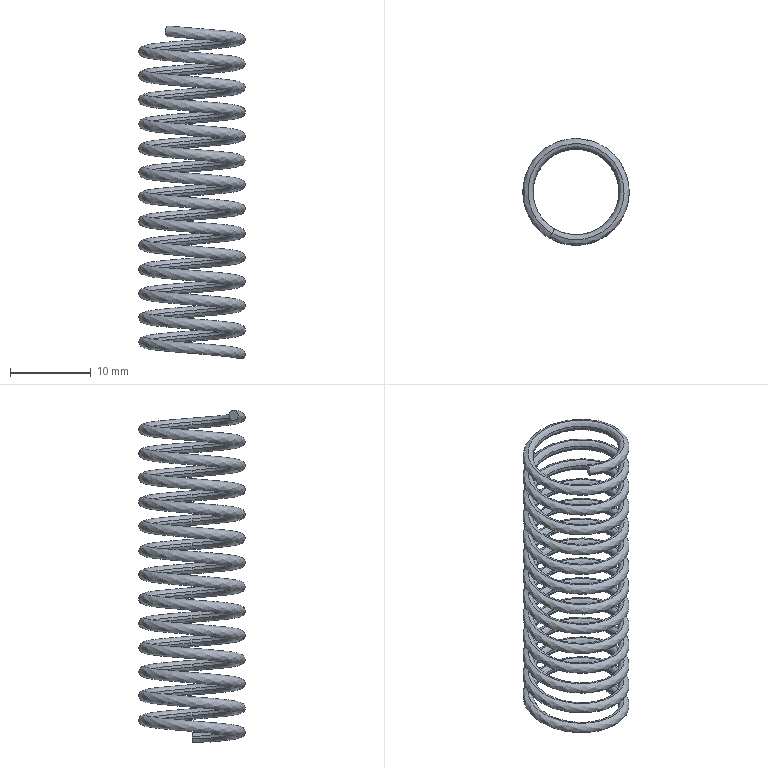Part | SolidWorks | features ICE 2, Helix 1, Sweep 1 | 1 solid | 34 faces | box 13.2 x 13.2 x 41.299 mm | volume 661.875 mm3 | cylinder 27 | plane 4 | spline 3 | commonest cylinder face diameters 10.65 x27